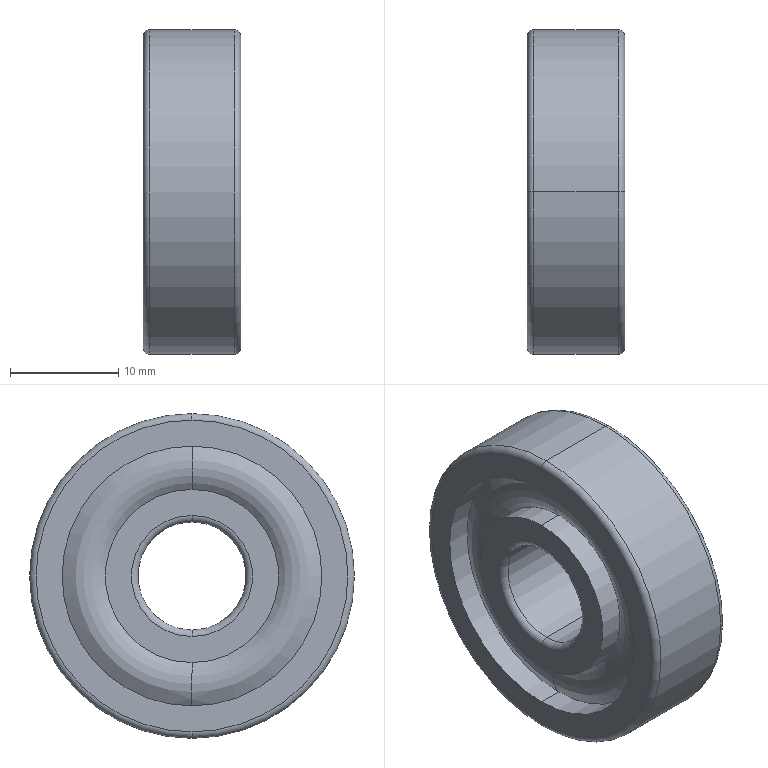Part | STEP file | radial ball bearing_68_skf_SKF - 6200 - 8,SI,NC,8_68 | 1 solid | 28 faces | box 9 x 30 x 30 mm | volume 4761 mm3 | torus 12 | cylinder 12 | plane 4 | commonest cylinder face diameters 16 x4 24 x4 10 x2 30 x2
STEP:
#1=CARTESIAN_POINT('',(-4.5,0.,-14.4));
#2=VERTEX_POINT('',#1);
#3=CARTESIAN_POINT('',(-4.5,0.,14.4));
#4=VERTEX_POINT('',#3);
#5=CARTESIAN_POINT('',(-4.5,0.,0.));
#6=DIRECTION('',(1.,0.,0.));
#7=DIRECTION('',(0.,0.,-1.));
#8=AXIS2_PLACEMENT_3D('',#5,#6,#7);
#9=CIRCLE('',#8,14.4);
#10=EDGE_CURVE('',#2,#4,#9,.T.);
#11=ORIENTED_EDGE('',*,*,#10,.T.);
#12=CARTESIAN_POINT('',(-3.9,0.,15.));
#13=VERTEX_POINT('',#12);
#14=CARTESIAN_POINT('',(-3.9,0.,14.4));
#15=DIRECTION('',(0.,1.,0.));
#16=DIRECTION('',(0.,0.,1.));
#17=AXIS2_PLACEMENT_3D('',#14,#15,#16);
#18=CIRCLE('',#17,0.6);
#19=EDGE_CURVE('',#4,#13,#18,.T.);
#20=ORIENTED_EDGE('',*,*,#19,.T.);
#21=CARTESIAN_POINT('',(-3.9,0.,-15.));
#22=VERTEX_POINT('',#21);
#23=CARTESIAN_POINT('',(-3.9,0.,0.));
#24=DIRECTION('',(1.,0.,0.));
#25=DIRECTION('',(0.,0.,-1.));
#26=AXIS2_PLACEMENT_3D('',#23,#24,#25);
#27=CIRCLE('',#26,15.);
#28=EDGE_CURVE('',#22,#13,#27,.T.);
#29=ORIENTED_EDGE('',*,*,#28,.F.);
#30=CARTESIAN_POINT('',(-3.9,0.,-14.4));
#31=DIRECTION('',(0.,-1.,0.));
#32=DIRECTION('',(0.,0.,-1.));
#33=AXIS2_PLACEMENT_3D('',#30,#31,#32);
#34=CIRCLE('',#33,0.6);
#35=EDGE_CURVE('',#2,#22,#34,.T.);
#36=ORIENTED_EDGE('',*,*,#35,.F.);
#37=EDGE_LOOP('',(#11,#20,#29,#36));
#38=FACE_OUTER_BOUND('',#37,.T.);
#39=CARTESIAN_POINT('',(-3.9,0.,0.));
#40=DIRECTION('',(1.,0.,0.));
#41=DIRECTION('',(0.,0.,-1.));
#42=AXIS2_PLACEMENT_3D('',#39,#40,#41);
#43=TOROIDAL_SURFACE('',#42,14.4,0.6);
#44=ADVANCED_FACE('',(#38),#43,.T.);
#45=ORIENTED_EDGE('',*,*,#28,.T.);
#46=CARTESIAN_POINT('',(3.9,0.,15.));
#47=VERTEX_POINT('',#46);
#48=CARTESIAN_POINT('',(-20.637,0.,15.));
#49=DIRECTION('',(1.,0.,0.));
#50=VECTOR('',#49,1000.);
#51=LINE('',#48,#50);
#52=EDGE_CURVE('',#13,#47,#51,.T.);
#53=ORIENTED_EDGE('',*,*,#52,.T.);
#54=CARTESIAN_POINT('',(3.9,0.,-15.));
#55=VERTEX_POINT('',#54);
#56=CARTESIAN_POINT('',(3.9,0.,0.));
#57=DIRECTION('',(1.,0.,0.));
#58=DIRECTION('',(0.,0.,-1.));
#59=AXIS2_PLACEMENT_3D('',#56,#57,#58);
#60=CIRCLE('',#59,15.);
#61=EDGE_CURVE('',#55,#47,#60,.T.);
#62=ORIENTED_EDGE('',*,*,#61,.F.);
#63=CARTESIAN_POINT('',(-20.637,0.,-15.));
#64=DIRECTION('',(1.,0.,0.));
#65=VECTOR('',#64,1000.);
#66=LINE('',#63,#65);
#67=EDGE_CURVE('',#22,#55,#66,.T.);
#68=ORIENTED_EDGE('',*,*,#67,.F.);
#69=EDGE_LOOP('',(#45,#53,#62,#68));
#70=FACE_OUTER_BOUND('',#69,.T.);
#71=CARTESIAN_POINT('',(-20.637,0.,0.));
#72=DIRECTION('',(1.,0.,0.));
#73=DIRECTION('',(0.,0.,-1.));
#74=AXIS2_PLACEMENT_3D('',#71,#72,#73);
#75=CYLINDRICAL_SURFACE('',#74,15.);
#76=ADVANCED_FACE('',(#70),#75,.T.);
#77=ORIENTED_EDGE('',*,*,#61,.T.);
#78=CARTESIAN_POINT('',(4.5,0.,14.4));
#79=VERTEX_POINT('',#78);
#80=CARTESIAN_POINT('',(3.9,0.,14.4));
#81=DIRECTION('',(0.,1.,0.));
#82=DIRECTION('',(0.,0.,1.));
#83=AXIS2_PLACEMENT_3D('',#80,#81,#82);
#84=CIRCLE('',#83,0.6);
#85=EDGE_CURVE('',#47,#79,#84,.T.);
#86=ORIENTED_EDGE('',*,*,#85,.T.);
#87=CARTESIAN_POINT('',(4.5,0.,-14.4));
#88=VERTEX_POINT('',#87);
#89=CARTESIAN_POINT('',(4.5,0.,0.));
#90=DIRECTION('',(1.,0.,0.));
#91=DIRECTION('',(0.,0.,-1.));
#92=AXIS2_PLACEMENT_3D('',#89,#90,#91);
#93=CIRCLE('',#92,14.4);
#94=EDGE_CURVE('',#88,#79,#93,.T.);
#95=ORIENTED_EDGE('',*,*,#94,.F.);
#96=CARTESIAN_POINT('',(3.9,0.,-14.4));
#97=DIRECTION('',(0.,-1.,0.));
#98=DIRECTION('',(0.,0.,-1.));
#99=AXIS2_PLACEMENT_3D('',#96,#97,#98);
#100=CIRCLE('',#99,0.6);
#101=EDGE_CURVE('',#55,#88,#100,.T.);
#102=ORIENTED_EDGE('',*,*,#101,.F.);
#103=EDGE_LOOP('',(#77,#86,#95,#102));
#104=FACE_OUTER_BOUND('',#103,.T.);
#105=CARTESIAN_POINT('',(3.9,0.,0.));
#106=DIRECTION('',(1.,0.,0.));
#107=DIRECTION('',(0.,0.,-1.));
#108=AXIS2_PLACEMENT_3D('',#105,#106,#107);
#109=TOROIDAL_SURFACE('',#108,14.4,0.6);
#110=ADVANCED_FACE('',(#104),#109,.T.);
#111=CARTESIAN_POINT('',(-4.5,0.,12.));
#112=VERTEX_POINT('',#111);
#113=CARTESIAN_POINT('',(-4.5,0.,-12.));
#114=VERTEX_POINT('',#113);
#115=CARTESIAN_POINT('',(-4.5,0.,0.));
#116=DIRECTION('',(1.,0.,0.));
#117=DIRECTION('',(0.,0.,-1.));
#118=AXIS2_PLACEMENT_3D('',#115,#116,#117);
#119=CIRCLE('',#118,12.);
#120=EDGE_CURVE('',#112,#114,#119,.T.);
#121=ORIENTED_EDGE('',*,*,#120,.F.);
#122=CARTESIAN_POINT('',(-2.236,0.,12.));
#123=VERTEX_POINT('',#122);
#124=CARTESIAN_POINT('',(-20.637,0.,12.));
#125=DIRECTION('',(1.,0.,0.));
#126=VECTOR('',#125,1000.);
#127=LINE('',#124,#126);
#128=EDGE_CURVE('',#112,#123,#127,.T.);
#129=ORIENTED_EDGE('',*,*,#128,.T.);
#130=CARTESIAN_POINT('',(-2.236,0.,-12.));
#131=VERTEX_POINT('',#130);
#132=CARTESIAN_POINT('',(-2.236,0.,0.));
#133=DIRECTION('',(-1.,0.,0.));
#134=DIRECTION('',(0.,0.,-1.));
#135=AXIS2_PLACEMENT_3D('',#132,#133,#134);
#136=CIRCLE('',#135,12.);
#137=EDGE_CURVE('',#131,#123,#136,.T.);
#138=ORIENTED_EDGE('',*,*,#137,.F.);
#139=CARTESIAN_POINT('',(-20.637,0.,-12.));
#140=DIRECTION('',(1.,0.,0.));
#141=VECTOR('',#140,1000.);
#142=LINE('',#139,#141);
#143=EDGE_CURVE('',#114,#131,#142,.T.);
#144=ORIENTED_EDGE('',*,*,#143,.F.);
#145=EDGE_LOOP('',(#121,#129,#138,#144));
#146=FACE_OUTER_BOUND('',#145,.T.);
#147=CARTESIAN_POINT('',(-20.637,0.,0.));
#148=DIRECTION('',(1.,0.,0.));
#149=DIRECTION('',(0.,0.,-1.));
#150=AXIS2_PLACEMENT_3D('',#147,#148,#149);
#151=CYLINDRICAL_SURFACE('',#150,12.);
#152=ADVANCED_FACE('',(#146),#151,.F.);
#153=CARTESIAN_POINT('',(2.236,0.,12.));
#154=VERTEX_POINT('',#153);
#155=CARTESIAN_POINT('',(2.236,0.,-12.));
#156=VERTEX_POINT('',#155);
#157=CARTESIAN_POINT('',(2.236,0.,0.));
#158=DIRECTION('',(1.,0.,0.));
#159=DIRECTION('',(0.,0.,1.));
#160=AXIS2_PLACEMENT_3D('',#157,#158,#159);
#161=CIRCLE('',#160,12.);
#162=EDGE_CURVE('',#154,#156,#161,.T.);
#163=ORIENTED_EDGE('',*,*,#162,.F.);
#164=CARTESIAN_POINT('',(4.5,0.,12.));
#165=VERTEX_POINT('',#164);
#166=CARTESIAN_POINT('',(-20.637,0.,12.));
#167=DIRECTION('',(1.,0.,0.));
#168=VECTOR('',#167,1000.);
#169=LINE('',#166,#168);
#170=EDGE_CURVE('',#154,#165,#169,.T.);
#171=ORIENTED_EDGE('',*,*,#170,.T.);
#172=CARTESIAN_POINT('',(4.5,0.,-12.));
#173=VERTEX_POINT('',#172);
#174=CARTESIAN_POINT('',(4.5,0.,0.));
#175=DIRECTION('',(1.,0.,0.));
#176=DIRECTION('',(0.,0.,-1.));
#177=AXIS2_PLACEMENT_3D('',#174,#175,#176);
#178=CIRCLE('',#177,12.);
#179=EDGE_CURVE('',#165,#173,#178,.T.);
#180=ORIENTED_EDGE('',*,*,#179,.T.);
#181=CARTESIAN_POINT('',(-20.637,0.,-12.));
#182=DIRECTION('',(1.,0.,0.));
#183=VECTOR('',#182,1000.);
#184=LINE('',#181,#183);
#185=EDGE_CURVE('',#156,#173,#184,.T.);
#186=ORIENTED_EDGE('',*,*,#185,.F.);
#187=EDGE_LOOP('',(#163,#171,#180,#186));
#188=FACE_OUTER_BOUND('',#187,.T.);
#189=CARTESIAN_POINT('',(-20.637,0.,0.));
#190=DIRECTION('',(1.,0.,0.));
#191=DIRECTION('',(0.,0.,-1.));
#192=AXIS2_PLACEMENT_3D('',#189,#190,#191);
#193=CYLINDRICAL_SURFACE('',#192,12.);
#194=ADVANCED_FACE('',(#188),#193,.F.);
#195=CARTESIAN_POINT('',(-2.236,0.,0.));
#196=DIRECTION('',(-1.,0.,0.));
#197=DIRECTION('',(0.,0.,-1.));
#198=AXIS2_PLACEMENT_3D('',#195,#196,#197);
#199=CIRCLE('',#198,12.);
#200=EDGE_CURVE('',#123,#131,#199,.T.);
#201=ORIENTED_EDGE('',*,*,#200,.T.);
#202=CARTESIAN_POINT('',(-2.236,0.,-8.));
#203=VERTEX_POINT('',#202);
#204=CARTESIAN_POINT('',(0.,0.,-10.));
#205=DIRECTION('',(0.,1.,0.));
#206=DIRECTION('',(0.,0.,1.));
#207=AXIS2_PLACEMENT_3D('',#204,#205,#206);
#208=CIRCLE('',#207,3.);
#209=EDGE_CURVE('',#131,#203,#208,.T.);
#210=ORIENTED_EDGE('',*,*,#209,.T.);
#211=CARTESIAN_POINT('',(-2.236,0.,8.));
#212=VERTEX_POINT('',#211);
#213=CARTESIAN_POINT('',(-2.236,0.,0.));
#214=DIRECTION('',(1.,0.,0.));
#215=DIRECTION('',(0.,0.,-1.));
#216=AXIS2_PLACEMENT_3D('',#213,#214,#215);
#217=CIRCLE('',#216,8.);
#218=EDGE_CURVE('',#203,#212,#217,.T.);
#219=ORIENTED_EDGE('',*,*,#218,.T.);
#220=CARTESIAN_POINT('',(0.,0.,10.));
#221=DIRECTION('',(0.,-1.,0.));
#222=DIRECTION('',(0.,0.,-1.));
#223=AXIS2_PLACEMENT_3D('',#220,#221,#222);
#224=CIRCLE('',#223,3.);
#225=EDGE_CURVE('',#123,#212,#224,.T.);
#226=ORIENTED_EDGE('',*,*,#225,.F.);
#227=EDGE_LOOP('',(#201,#210,#219,#226));
#228=FACE_OUTER_BOUND('',#227,.T.);
#229=CARTESIAN_POINT('',(0.,0.,0.));
#230=DIRECTION('',(-1.,0.,0.));
#231=DIRECTION('',(0.,0.,1.));
#232=AXIS2_PLACEMENT_3D('',#229,#230,#231);
#233=TOROIDAL_SURFACE('',#232,10.,3.);
#234=ADVANCED_FACE('',(#228),#233,.T.);
#235=CARTESIAN_POINT('',(-3.9,0.,-5.));
#236=VERTEX_POINT('',#235);
#237=CARTESIAN_POINT('',(-3.9,0.,5.));
#238=VERTEX_POINT('',#237);
#239=CARTESIAN_POINT('',(-3.9,0.,0.));
#240=DIRECTION('',(1.,0.,0.));
#241=DIRECTION('',(0.,0.,-1.));
#242=AXIS2_PLACEMENT_3D('',#239,#240,#241);
#243=CIRCLE('',#242,5.);
#244=EDGE_CURVE('',#236,#238,#243,.T.);
#245=ORIENTED_EDGE('',*,*,#244,.T.);
#246=CARTESIAN_POINT('',(-4.5,0.,5.6));
#247=VERTEX_POINT('',#246);
#248=CARTESIAN_POINT('',(-3.9,0.,5.6));
#249=DIRECTION('',(0.,1.,0.));
#250=DIRECTION('',(0.,0.,1.));
#251=AXIS2_PLACEMENT_3D('',#248,#249,#250);
#252=CIRCLE('',#251,0.6);
#253=EDGE_CURVE('',#238,#247,#252,.T.);
#254=ORIENTED_EDGE('',*,*,#253,.T.);
#255=CARTESIAN_POINT('',(-4.5,0.,-5.6));
#256=VERTEX_POINT('',#255);
#257=CARTESIAN_POINT('',(-4.5,0.,0.));
#258=DIRECTION('',(1.,0.,0.));
#259=DIRECTION('',(0.,0.,-1.));
#260=AXIS2_PLACEMENT_3D('',#257,#258,#259);
#261=CIRCLE('',#260,5.6);
#262=EDGE_CURVE('',#256,#247,#261,.T.);
#263=ORIENTED_EDGE('',*,*,#262,.F.);
#264=CARTESIAN_POINT('',(-3.9,0.,-5.6));
#265=DIRECTION('',(0.,-1.,0.));
#266=DIRECTION('',(0.,0.,-1.));
#267=AXIS2_PLACEMENT_3D('',#264,#265,#266);
#268=CIRCLE('',#267,0.6);
#269=EDGE_CURVE('',#236,#256,#268,.T.);
#270=ORIENTED_EDGE('',*,*,#269,.F.);
#271=EDGE_LOOP('',(#245,#254,#263,#270));
#272=FACE_OUTER_BOUND('',#271,.T.);
#273=CARTESIAN_POINT('',(-3.9,0.,0.));
#274=DIRECTION('',(1.,0.,0.));
#275=DIRECTION('',(0.,0.,-1.));
#276=AXIS2_PLACEMENT_3D('',#273,#274,#275);
#277=TOROIDAL_SURFACE('',#276,5.6,0.6);
#278=ADVANCED_FACE('',(#272),#277,.T.);
#279=CARTESIAN_POINT('',(-3.9,0.,0.));
#280=DIRECTION('',(1.,0.,0.));
#281=DIRECTION('',(0.,0.,-1.));
#282=AXIS2_PLACEMENT_3D('',#279,#280,#281);
#283=CIRCLE('',#282,5.);
#284=EDGE_CURVE('',#238,#236,#283,.T.);
#285=ORIENTED_EDGE('',*,*,#284,.F.);
#286=CARTESIAN_POINT('',(3.9,0.,5.));
#287=VERTEX_POINT('',#286);
#288=CARTESIAN_POINT('',(-20.637,0.,5.));
#289=DIRECTION('',(1.,0.,0.));
#290=VECTOR('',#289,1000.);
#291=LINE('',#288,#290);
#292=EDGE_CURVE('',#238,#287,#291,.T.);
#293=ORIENTED_EDGE('',*,*,#292,.T.);
#294=CARTESIAN_POINT('',(3.9,0.,-5.));
#295=VERTEX_POINT('',#294);
#296=CARTESIAN_POINT('',(3.9,0.,0.));
#297=DIRECTION('',(1.,0.,0.));
#298=DIRECTION('',(0.,0.,-1.));
#299=AXIS2_PLACEMENT_3D('',#296,#297,#298);
#300=CIRCLE('',#299,5.);
#301=EDGE_CURVE('',#287,#295,#300,.T.);
#302=ORIENTED_EDGE('',*,*,#301,.T.);
#303=CARTESIAN_POINT('',(-20.637,0.,-5.));
#304=DIRECTION('',(1.,0.,0.));
#305=VECTOR('',#304,1000.);
#306=LINE('',#303,#305);
#307=EDGE_CURVE('',#236,#295,#306,.T.);
#308=ORIENTED_EDGE('',*,*,#307,.F.);
#309=EDGE_LOOP('',(#285,#293,#302,#308));
#310=FACE_OUTER_BOUND('',#309,.T.);
#311=CARTESIAN_POINT('',(-20.637,0.,0.));
#312=DIRECTION('',(1.,0.,0.));
#313=DIRECTION('',(0.,0.,-1.));
#314=AXIS2_PLACEMENT_3D('',#311,#312,#313);
#315=CYLINDRICAL_SURFACE('',#314,5.);
#316=ADVANCED_FACE('',(#310),#315,.F.);
#317=CARTESIAN_POINT('',(4.5,0.,-5.6));
#318=VERTEX_POINT('',#317);
#319=CARTESIAN_POINT('',(4.5,0.,5.6));
#320=VERTEX_POINT('',#319);
#321=CARTESIAN_POINT('',(4.5,0.,0.));
#322=DIRECTION('',(1.,0.,0.));
#323=DIRECTION('',(0.,0.,-1.));
#324=AXIS2_PLACEMENT_3D('',#321,#322,#323);
#325=CIRCLE('',#324,5.6);
#326=EDGE_CURVE('',#318,#320,#325,.T.);
#327=ORIENTED_EDGE('',*,*,#326,.T.);
#328=CARTESIAN_POINT('',(3.9,0.,5.6));
#329=DIRECTION('',(0.,1.,0.));
#330=DIRECTION('',(0.,0.,1.));
#331=AXIS2_PLACEMENT_3D('',#328,#329,#330);
#332=CIRCLE('',#331,0.6);
#333=EDGE_CURVE('',#320,#287,#332,.T.);
#334=ORIENTED_EDGE('',*,*,#333,.T.);
#335=CARTESIAN_POINT('',(3.9,0.,0.));
#336=DIRECTION('',(1.,0.,0.));
#337=DIRECTION('',(0.,0.,-1.));
#338=AXIS2_PLACEMENT_3D('',#335,#336,#337);
#339=CIRCLE('',#338,5.);
#340=EDGE_CURVE('',#295,#287,#339,.T.);
#341=ORIENTED_EDGE('',*,*,#340,.F.);
#342=CARTESIAN_POINT('',(3.9,0.,-5.6));
#343=DIRECTION('',(0.,-1.,0.));
#344=DIRECTION('',(0.,0.,-1.));
#345=AXIS2_PLACEMENT_3D('',#342,#343,#344);
#346=CIRCLE('',#345,0.6);
#347=EDGE_CURVE('',#318,#295,#346,.T.);
#348=ORIENTED_EDGE('',*,*,#347,.F.);
#349=EDGE_LOOP('',(#327,#334,#341,#348));
#350=FACE_OUTER_BOUND('',#349,.T.);
#351=CARTESIAN_POINT('',(3.9,0.,0.));
#352=DIRECTION('',(1.,0.,0.));
#353=DIRECTION('',(0.,0.,-1.));
#354=AXIS2_PLACEMENT_3D('',#351,#352,#353);
#355=TOROIDAL_SURFACE('',#354,5.6,0.6);
#356=ADVANCED_FACE('',(#350),#355,.T.);
#357=CARTESIAN_POINT('',(-4.5,0.,-8.));
#358=VERTEX_POINT('',#357);
#359=CARTESIAN_POINT('',(-4.5,0.,8.));
#360=VERTEX_POINT('',#359);
#361=CARTESIAN_POINT('',(-4.5,0.,0.));
#362=DIRECTION('',(1.,0.,0.));
#363=DIRECTION('',(0.,0.,-1.));
#364=AXIS2_PLACEMENT_3D('',#361,#362,#363);
#365=CIRCLE('',#364,8.);
#366=EDGE_CURVE('',#358,#360,#365,.T.);
#367=ORIENTED_EDGE('',*,*,#366,.T.);
#368=CARTESIAN_POINT('',(-20.637,0.,8.));
#369=DIRECTION('',(1.,0.,0.));
#370=VECTOR('',#369,1000.);
#371=LINE('',#368,#370);
#372=EDGE_CURVE('',#360,#212,#371,.T.);
#373=ORIENTED_EDGE('',*,*,#372,.T.);
#374=ORIENTED_EDGE('',*,*,#218,.F.);
#375=CARTESIAN_POINT('',(-20.637,0.,-8.));
#376=DIRECTION('',(1.,0.,0.));
#377=VECTOR('',#376,1000.);
#378=LINE('',#375,#377);
#379=EDGE_CURVE('',#358,#203,#378,.T.);
#380=ORIENTED_EDGE('',*,*,#379,.F.);
#381=EDGE_LOOP('',(#367,#373,#374,#380));
#382=FACE_OUTER_BOUND('',#381,.T.);
#383=CARTESIAN_POINT('',(-20.637,0.,0.));
#384=DIRECTION('',(1.,0.,0.));
#385=DIRECTION('',(0.,0.,-1.));
#386=AXIS2_PLACEMENT_3D('',#383,#384,#385);
#387=CYLINDRICAL_SURFACE('',#386,8.);
#388=ADVANCED_FACE('',(#382),#387,.T.);
#389=CARTESIAN_POINT('',(2.236,0.,8.));
#390=VERTEX_POINT('',#389);
#391=CARTESIAN_POINT('',(2.236,0.,-8.));
#392=VERTEX_POINT('',#391);
#393=CARTESIAN_POINT('',(2.236,0.,0.));
#394=DIRECTION('',(-1.,0.,0.));
#395=DIRECTION('',(0.,0.,1.));
#396=AXIS2_PLACEMENT_3D('',#393,#394,#395);
#397=CIRCLE('',#396,8.);
#398=EDGE_CURVE('',#390,#392,#397,.T.);
#399=ORIENTED_EDGE('',*,*,#398,.F.);
#400=CARTESIAN_POINT('',(4.5,0.,8.));
#401=VERTEX_POINT('',#400);
#402=CARTESIAN_POINT('',(-20.637,0.,8.));
#403=DIRECTION('',(1.,0.,0.));
#404=VECTOR('',#403,1000.);
#405=LINE('',#402,#404);
#406=EDGE_CURVE('',#390,#401,#405,.T.);
#407=ORIENTED_EDGE('',*,*,#406,.T.);
#408=CARTESIAN_POINT('',(4.5,0.,-8.));
#409=VERTEX_POINT('',#408);
#410=CARTESIAN_POINT('',(4.5,0.,0.));
#411=DIRECTION('',(1.,0.,0.));
#412=DIRECTION('',(0.,0.,-1.));
#413=AXIS2_PLACEMENT_3D('',#410,#411,#412);
#414=CIRCLE('',#413,8.);
#415=EDGE_CURVE('',#409,#401,#414,.T.);
#416=ORIENTED_EDGE('',*,*,#415,.F.);
#417=CARTESIAN_POINT('',(-20.637,0.,-8.));
#418=DIRECTION('',(1.,0.,0.));
#419=VECTOR('',#418,1000.);
#420=LINE('',#417,#419);
#421=EDGE_CURVE('',#392,#409,#420,.T.);
#422=ORIENTED_EDGE('',*,*,#421,.F.);
#423=EDGE_LOOP('',(#399,#407,#416,#422));
#424=FACE_OUTER_BOUND('',#423,.T.);
#425=CARTESIAN_POINT('',(-20.637,0.,0.));
#426=DIRECTION('',(1.,0.,0.));
#427=DIRECTION('',(0.,0.,-1.));
#428=AXIS2_PLACEMENT_3D('',#425,#426,#427);
#429=CYLINDRICAL_SURFACE('',#428,8.);
#430=ADVANCED_FACE('',(#424),#429,.T.);
#431=ORIENTED_EDGE('',*,*,#398,.T.);
#432=CARTESIAN_POINT('',(0.,0.,-10.));
#433=DIRECTION('',(0.,1.,0.));
#434=DIRECTION('',(0.,0.,1.));
#435=AXIS2_PLACEMENT_3D('',#432,#433,#434);
#436=CIRCLE('',#435,3.);
#437=EDGE_CURVE('',#392,#156,#436,.T.);
#438=ORIENTED_EDGE('',*,*,#437,.T.);
#439=CARTESIAN_POINT('',(2.236,0.,0.));
#440=DIRECTION('',(1.,0.,0.));
#441=DIRECTION('',(0.,0.,1.));
#442=AXIS2_PLACEMENT_3D('',#439,#440,#441);
#443=CIRCLE('',#442,12.);
#444=EDGE_CURVE('',#156,#154,#443,.T.);
#445=ORIENTED_EDGE('',*,*,#444,.T.);
#446=CARTESIAN_POINT('',(0.,0.,10.));
#447=DIRECTION('',(0.,-1.,0.));
#448=DIRECTION('',(0.,0.,-1.));
#449=AXIS2_PLACEMENT_3D('',#446,#447,#448);
#450=CIRCLE('',#449,3.);
#451=EDGE_CURVE('',#390,#154,#450,.T.);
#452=ORIENTED_EDGE('',*,*,#451,.F.);
#453=EDGE_LOOP('',(#431,#438,#445,#452));
#454=FACE_OUTER_BOUND('',#453,.T.);
#455=CARTESIAN_POINT('',(0.,0.,0.));
#456=DIRECTION('',(-1.,0.,0.));
#457=DIRECTION('',(0.,0.,1.));
#458=AXIS2_PLACEMENT_3D('',#455,#456,#457);
#459=TOROIDAL_SURFACE('',#458,10.,3.);
#460=ADVANCED_FACE('',(#454),#459,.T.);
#461=ORIENTED_EDGE('',*,*,#437,.F.);
#462=CARTESIAN_POINT('',(2.236,0.,0.));
#463=DIRECTION('',(-1.,0.,0.));
#464=DIRECTION('',(0.,0.,1.));
#465=AXIS2_PLACEMENT_3D('',#462,#463,#464);
#466=CIRCLE('',#465,8.);
#467=EDGE_CURVE('',#392,#390,#466,.T.);
#468=ORIENTED_EDGE('',*,*,#467,.T.);
#469=ORIENTED_EDGE('',*,*,#451,.T.);
#470=ORIENTED_EDGE('',*,*,#162,.T.);
#471=EDGE_LOOP('',(#461,#468,#469,#470));
#472=FACE_OUTER_BOUND('',#471,.T.);
#473=CARTESIAN_POINT('',(0.,0.,0.));
#474=DIRECTION('',(-1.,0.,0.));
#475=DIRECTION('',(0.,0.,1.));
#476=AXIS2_PLACEMENT_3D('',#473,#474,#475);
#477=TOROIDAL_SURFACE('',#476,10.,3.);
#478=ADVANCED_FACE('',(#472),#477,.T.);
#479=ORIENTED_EDGE('',*,*,#406,.F.);
#480=ORIENTED_EDGE('',*,*,#467,.F.);
#481=ORIENTED_EDGE('',*,*,#421,.T.);
#482=CARTESIAN_POINT('',(4.5,0.,0.));
#483=DIRECTION('',(1.,0.,0.));
#484=DIRECTION('',(0.,0.,-1.));
#485=AXIS2_PLACEMENT_3D('',#482,#483,#484);
#486=CIRCLE('',#485,8.);
#487=EDGE_CURVE('',#401,#409,#486,.T.);
#488=ORIENTED_EDGE('',*,*,#487,.F.);
#489=EDGE_LOOP('',(#479,#480,#481,#488));
#490=FACE_OUTER_BOUND('',#489,.T.);
#491=CARTESIAN_POINT('',(-20.637,0.,0.));
#492=DIRECTION('',(1.,0.,0.));
#493=DIRECTION('',(0.,0.,-1.));
#494=AXIS2_PLACEMENT_3D('',#491,#492,#493);
#495=CYLINDRICAL_SURFACE('',#494,8.);
#496=ADVANCED_FACE('',(#490),#495,.T.);
#497=ORIENTED_EDGE('',*,*,#372,.F.);
#498=CARTESIAN_POINT('',(-4.5,0.,0.));
#499=DIRECTION('',(1.,0.,0.));
#500=DIRECTION('',(0.,0.,-1.));
#501=AXIS2_PLACEMENT_3D('',#498,#499,#500);
#502=CIRCLE('',#501,8.);
#503=EDGE_CURVE('',#360,#358,#502,.T.);
#504=ORIENTED_EDGE('',*,*,#503,.T.);
#505=ORIENTED_EDGE('',*,*,#379,.T.);
#506=CARTESIAN_POINT('',(-2.236,0.,0.));
#507=DIRECTION('',(1.,0.,0.));
#508=DIRECTION('',(0.,0.,-1.));
#509=AXIS2_PLACEMENT_3D('',#506,#507,#508);
#510=CIRCLE('',#509,8.);
#511=EDGE_CURVE('',#212,#203,#510,.T.);
#512=ORIENTED_EDGE('',*,*,#511,.F.);
#513=EDGE_LOOP('',(#497,#504,#505,#512));
#514=FACE_OUTER_BOUND('',#513,.T.);
#515=CARTESIAN_POINT('',(-20.637,0.,0.));
#516=DIRECTION('',(1.,0.,0.));
#517=DIRECTION('',(0.,0.,-1.));
#518=AXIS2_PLACEMENT_3D('',#515,#516,#517);
#519=CYLINDRICAL_SURFACE('',#518,8.);
#520=ADVANCED_FACE('',(#514),#519,.T.);
#521=ORIENTED_EDGE('',*,*,#415,.T.);
#522=ORIENTED_EDGE('',*,*,#487,.T.);
#523=EDGE_LOOP('',(#521,#522));
#524=FACE_OUTER_BOUND('',#523,.T.);
#525=ORIENTED_EDGE('',*,*,#326,.F.);
#526=CARTESIAN_POINT('',(4.5,0.,0.));
#527=DIRECTION('',(1.,0.,0.));
#528=DIRECTION('',(0.,0.,-1.));
#529=AXIS2_PLACEMENT_3D('',#526,#527,#528);
#530=CIRCLE('',#529,5.6);
#531=EDGE_CURVE('',#320,#318,#530,.T.);
#532=ORIENTED_EDGE('',*,*,#531,.F.);
#533=EDGE_LOOP('',(#525,#532));
#534=FACE_BOUND('',#533,.T.);
#535=CARTESIAN_POINT('',(4.5,5.6,0.));
#536=DIRECTION('',(1.,0.,0.));
#537=DIRECTION('',(0.,0.,-1.));
#538=AXIS2_PLACEMENT_3D('',#535,#536,#537);
#539=PLANE('',#538);
#540=ADVANCED_FACE('',(#524,#534),#539,.T.);
#541=ORIENTED_EDGE('',*,*,#333,.F.);
#542=ORIENTED_EDGE('',*,*,#531,.T.);
#543=ORIENTED_EDGE('',*,*,#347,.T.);
#544=ORIENTED_EDGE('',*,*,#301,.F.);
#545=EDGE_LOOP('',(#541,#542,#543,#544));
#546=FACE_OUTER_BOUND('',#545,.T.);
#547=CARTESIAN_POINT('',(3.9,0.,0.));
#548=DIRECTION('',(1.,0.,0.));
#549=DIRECTION('',(0.,0.,-1.));
#550=AXIS2_PLACEMENT_3D('',#547,#548,#549);
#551=TOROIDAL_SURFACE('',#550,5.6,0.6);
#552=ADVANCED_FACE('',(#546),#551,.T.);
#553=ORIENTED_EDGE('',*,*,#292,.F.);
#554=ORIENTED_EDGE('',*,*,#244,.F.);
#555=ORIENTED_EDGE('',*,*,#307,.T.);
#556=ORIENTED_EDGE('',*,*,#340,.T.);
#557=EDGE_LOOP('',(#553,#554,#555,#556));
#558=FACE_OUTER_BOUND('',#557,.T.);
#559=CARTESIAN_POINT('',(-20.637,0.,0.));
#560=DIRECTION('',(1.,0.,0.));
#561=DIRECTION('',(0.,0.,-1.));
#562=AXIS2_PLACEMENT_3D('',#559,#560,#561);
#563=CYLINDRICAL_SURFACE('',#562,5.);
#564=ADVANCED_FACE('',(#558),#563,.F.);
#565=ORIENTED_EDGE('',*,*,#253,.F.);
#566=ORIENTED_EDGE('',*,*,#284,.T.);
#567=ORIENTED_EDGE('',*,*,#269,.T.);
#568=CARTESIAN_POINT('',(-4.5,0.,0.));
#569=DIRECTION('',(1.,0.,0.));
#570=DIRECTION('',(0.,0.,-1.));
#571=AXIS2_PLACEMENT_3D('',#568,#569,#570);
#572=CIRCLE('',#571,5.6);
#573=EDGE_CURVE('',#247,#256,#572,.T.);
#574=ORIENTED_EDGE('',*,*,#573,.F.);
#575=EDGE_LOOP('',(#565,#566,#567,#574));
#576=FACE_OUTER_BOUND('',#575,.T.);
#577=CARTESIAN_POINT('',(-3.9,0.,0.));
#578=DIRECTION('',(1.,0.,0.));
#579=DIRECTION('',(0.,0.,-1.));
#580=AXIS2_PLACEMENT_3D('',#577,#578,#579);
#581=TOROIDAL_SURFACE('',#580,5.6,0.6);
#582=ADVANCED_FACE('',(#576),#581,.T.);
#583=ORIENTED_EDGE('',*,*,#262,.T.);
#584=ORIENTED_EDGE('',*,*,#573,.T.);
#585=EDGE_LOOP('',(#583,#584));
#586=FACE_BOUND('',#585,.T.);
#587=ORIENTED_EDGE('',*,*,#366,.F.);
#588=ORIENTED_EDGE('',*,*,#503,.F.);
#589=EDGE_LOOP('',(#587,#588));
#590=FACE_OUTER_BOUND('',#589,.T.);
#591=CARTESIAN_POINT('',(-4.5,8.,0.));
#592=DIRECTION('',(-1.,0.,0.));
#593=DIRECTION('',(0.,0.,1.));
#594=AXIS2_PLACEMENT_3D('',#591,#592,#593);
#595=PLANE('',#594);
#596=ADVANCED_FACE('',(#586,#590),#595,.T.);
#597=ORIENTED_EDGE('',*,*,#209,.F.);
#598=ORIENTED_EDGE('',*,*,#137,.T.);
#599=ORIENTED_EDGE('',*,*,#225,.T.);
#600=ORIENTED_EDGE('',*,*,#511,.T.);
#601=EDGE_LOOP('',(#597,#598,#599,#600));
#602=FACE_OUTER_BOUND('',#601,.T.);
#603=CARTESIAN_POINT('',(0.,0.,0.));
#604=DIRECTION('',(-1.,0.,0.));
#605=DIRECTION('',(0.,0.,1.));
#606=AXIS2_PLACEMENT_3D('',#603,#604,#605);
#607=TOROIDAL_SURFACE('',#606,10.,3.);
#608=ADVANCED_FACE('',(#602),#607,.T.);
#609=ORIENTED_EDGE('',*,*,#170,.F.);
#610=ORIENTED_EDGE('',*,*,#444,.F.);
#611=ORIENTED_EDGE('',*,*,#185,.T.);
#612=CARTESIAN_POINT('',(4.5,0.,0.));
#613=DIRECTION('',(1.,0.,0.));
#614=DIRECTION('',(0.,0.,-1.));
#615=AXIS2_PLACEMENT_3D('',#612,#613,#614);
#616=CIRCLE('',#615,12.);
#617=EDGE_CURVE('',#173,#165,#616,.T.);
#618=ORIENTED_EDGE('',*,*,#617,.T.);
#619=EDGE_LOOP('',(#609,#610,#611,#618));
#620=FACE_OUTER_BOUND('',#619,.T.);
#621=CARTESIAN_POINT('',(-20.637,0.,0.));
#622=DIRECTION('',(1.,0.,0.));
#623=DIRECTION('',(0.,0.,-1.));
#624=AXIS2_PLACEMENT_3D('',#621,#622,#623);
#625=CYLINDRICAL_SURFACE('',#624,12.);
#626=ADVANCED_FACE('',(#620),#625,.F.);
#627=ORIENTED_EDGE('',*,*,#128,.F.);
#628=CARTESIAN_POINT('',(-4.5,0.,0.));
#629=DIRECTION('',(1.,0.,0.));
#630=DIRECTION('',(0.,0.,-1.));
#631=AXIS2_PLACEMENT_3D('',#628,#629,#630);
#632=CIRCLE('',#631,12.);
#633=EDGE_CURVE('',#114,#112,#632,.T.);
#634=ORIENTED_EDGE('',*,*,#633,.F.);
#635=ORIENTED_EDGE('',*,*,#143,.T.);
#636=ORIENTED_EDGE('',*,*,#200,.F.);
#637=EDGE_LOOP('',(#627,#634,#635,#636));
#638=FACE_OUTER_BOUND('',#637,.T.);
#639=CARTESIAN_POINT('',(-20.637,0.,0.));
#640=DIRECTION('',(1.,0.,0.));
#641=DIRECTION('',(0.,0.,-1.));
#642=AXIS2_PLACEMENT_3D('',#639,#640,#641);
#643=CYLINDRICAL_SURFACE('',#642,12.);
#644=ADVANCED_FACE('',(#638),#643,.F.);
#645=ORIENTED_EDGE('',*,*,#94,.T.);
#646=CARTESIAN_POINT('',(4.5,0.,0.));
#647=DIRECTION('',(1.,0.,0.));
#648=DIRECTION('',(0.,0.,-1.));
#649=AXIS2_PLACEMENT_3D('',#646,#647,#648);
#650=CIRCLE('',#649,14.4);
#651=EDGE_CURVE('',#79,#88,#650,.T.);
#652=ORIENTED_EDGE('',*,*,#651,.T.);
#653=EDGE_LOOP('',(#645,#652));
#654=FACE_OUTER_BOUND('',#653,.T.);
#655=ORIENTED_EDGE('',*,*,#617,.F.);
#656=ORIENTED_EDGE('',*,*,#179,.F.);
#657=EDGE_LOOP('',(#655,#656));
#658=FACE_BOUND('',#657,.T.);
#659=CARTESIAN_POINT('',(4.5,14.4,0.));
#660=DIRECTION('',(1.,0.,0.));
#661=DIRECTION('',(0.,0.,-1.));
#662=AXIS2_PLACEMENT_3D('',#659,#660,#661);
#663=PLANE('',#662);
#664=ADVANCED_FACE('',(#654,#658),#663,.T.);
#665=ORIENTED_EDGE('',*,*,#85,.F.);
#666=CARTESIAN_POINT('',(3.9,0.,0.));
#667=DIRECTION('',(1.,0.,0.));
#668=DIRECTION('',(0.,0.,-1.));
#669=AXIS2_PLACEMENT_3D('',#666,#667,#668);
#670=CIRCLE('',#669,15.);
#671=EDGE_CURVE('',#47,#55,#670,.T.);
#672=ORIENTED_EDGE('',*,*,#671,.T.);
#673=ORIENTED_EDGE('',*,*,#101,.T.);
#674=ORIENTED_EDGE('',*,*,#651,.F.);
#675=EDGE_LOOP('',(#665,#672,#673,#674));
#676=FACE_OUTER_BOUND('',#675,.T.);
#677=CARTESIAN_POINT('',(3.9,0.,0.));
#678=DIRECTION('',(1.,0.,0.));
#679=DIRECTION('',(0.,0.,-1.));
#680=AXIS2_PLACEMENT_3D('',#677,#678,#679);
#681=TOROIDAL_SURFACE('',#680,14.4,0.6);
#682=ADVANCED_FACE('',(#676),#681,.T.);
#683=ORIENTED_EDGE('',*,*,#52,.F.);
#684=CARTESIAN_POINT('',(-3.9,0.,0.));
#685=DIRECTION('',(1.,0.,0.));
#686=DIRECTION('',(0.,0.,-1.));
#687=AXIS2_PLACEMENT_3D('',#684,#685,#686);
#688=CIRCLE('',#687,15.);
#689=EDGE_CURVE('',#13,#22,#688,.T.);
#690=ORIENTED_EDGE('',*,*,#689,.T.);
#691=ORIENTED_EDGE('',*,*,#67,.T.);
#692=ORIENTED_EDGE('',*,*,#671,.F.);
#693=EDGE_LOOP('',(#683,#690,#691,#692));
#694=FACE_OUTER_BOUND('',#693,.T.);
#695=CARTESIAN_POINT('',(-20.637,0.,0.));
#696=DIRECTION('',(1.,0.,0.));
#697=DIRECTION('',(0.,0.,-1.));
#698=AXIS2_PLACEMENT_3D('',#695,#696,#697);
#699=CYLINDRICAL_SURFACE('',#698,15.);
#700=ADVANCED_FACE('',(#694),#699,.T.);
#701=ORIENTED_EDGE('',*,*,#19,.F.);
#702=CARTESIAN_POINT('',(-4.5,0.,0.));
#703=DIRECTION('',(1.,0.,0.));
#704=DIRECTION('',(0.,0.,-1.));
#705=AXIS2_PLACEMENT_3D('',#702,#703,#704);
#706=CIRCLE('',#705,14.4);
#707=EDGE_CURVE('',#4,#2,#706,.T.);
#708=ORIENTED_EDGE('',*,*,#707,.T.);
#709=ORIENTED_EDGE('',*,*,#35,.T.);
#710=ORIENTED_EDGE('',*,*,#689,.F.);
#711=EDGE_LOOP('',(#701,#708,#709,#710));
#712=FACE_OUTER_BOUND('',#711,.T.);
#713=CARTESIAN_POINT('',(-3.9,0.,0.));
#714=DIRECTION('',(1.,0.,0.));
#715=DIRECTION('',(0.,0.,-1.));
#716=AXIS2_PLACEMENT_3D('',#713,#714,#715);
#717=TOROIDAL_SURFACE('',#716,14.4,0.6);
#718=ADVANCED_FACE('',(#712),#717,.T.);
#719=ORIENTED_EDGE('',*,*,#633,.T.);
#720=ORIENTED_EDGE('',*,*,#120,.T.);
#721=EDGE_LOOP('',(#719,#720));
#722=FACE_BOUND('',#721,.T.);
#723=ORIENTED_EDGE('',*,*,#10,.F.);
#724=ORIENTED_EDGE('',*,*,#707,.F.);
#725=EDGE_LOOP('',(#723,#724));
#726=FACE_OUTER_BOUND('',#725,.T.);
#727=CARTESIAN_POINT('',(-4.5,12.,0.));
#728=DIRECTION('',(-1.,0.,0.));
#729=DIRECTION('',(0.,0.,1.));
#730=AXIS2_PLACEMENT_3D('',#727,#728,#729);
#731=PLANE('',#730);
#732=ADVANCED_FACE('',(#722,#726),#731,.T.);
#733=CLOSED_SHELL('',(#44,#76,#110,#152,#194,#234,#278,#316,#356,#388,#430,#460,#478,#496,#520,#540,#552,#564,#582,#596,#608,#626,#644,#664,#682,#700,#718,#732));
#734=MANIFOLD_SOLID_BREP('',#733);
#735=CARTESIAN_POINT('',(0.,0.,0.));
#736=DIRECTION('',(0.,0.,1.));
#737=DIRECTION('',(1.,0.,0.));
#738=AXIS2_PLACEMENT_3D('',#735,#736,#737);
#739=(LENGTH_UNIT()NAMED_UNIT(*)SI_UNIT(.MILLI.,.METRE.));
#740=UNCERTAINTY_MEASURE_WITH_UNIT(LENGTH_MEASURE(0.00001),#739,'','');
#741=(NAMED_UNIT(*)PLANE_ANGLE_UNIT()SI_UNIT($,.RADIAN.));
#742=(NAMED_UNIT(*)SI_UNIT($,.STERADIAN.)SOLID_ANGLE_UNIT());
#743=(GEOMETRIC_REPRESENTATION_CONTEXT(3)GLOBAL_UNCERTAINTY_ASSIGNED_CONTEXT((#740))GLOBAL_UNIT_ASSIGNED_CONTEXT((#739,#741,#742))REPRESENTATION_CONTEXT('',''));
#744=ADVANCED_BREP_SHAPE_REPRESENTATION('',(#734,#738),#743);